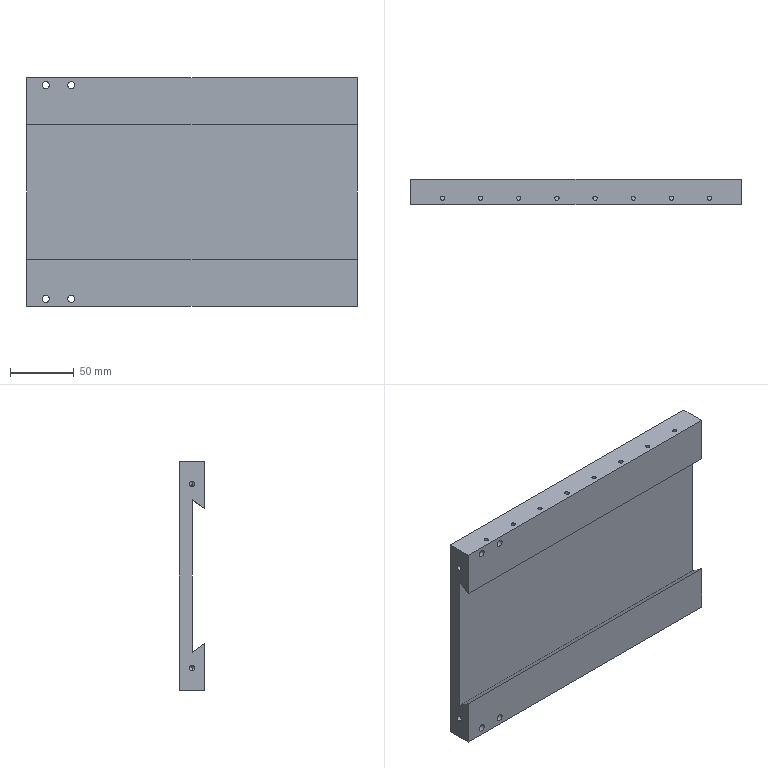Part | STEP file | 06-32 Up-down adjusting dovetail groove | 1 solid | 54 faces | box 260 x 20 x 180 mm | volume 636123 mm3 | cylinder 36 | plane 14 | cone 4 | commonest cylinder face diameters 3.3 x16 5.5 x8 10 x8 4.2 x4